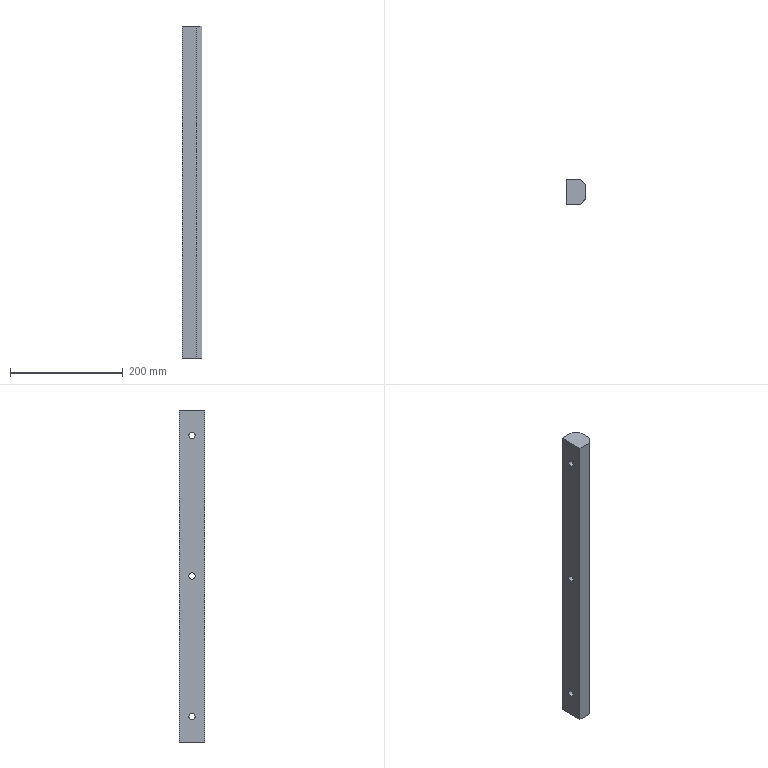Part | STEP file | PN_0057_protective stopper | 1 solid | 23 faces | box 35 x 45 x 590 mm | volume 854484 mm3 | cylinder 12 | plane 11 | commonest cylinder face diameters 11 x6 18 x6